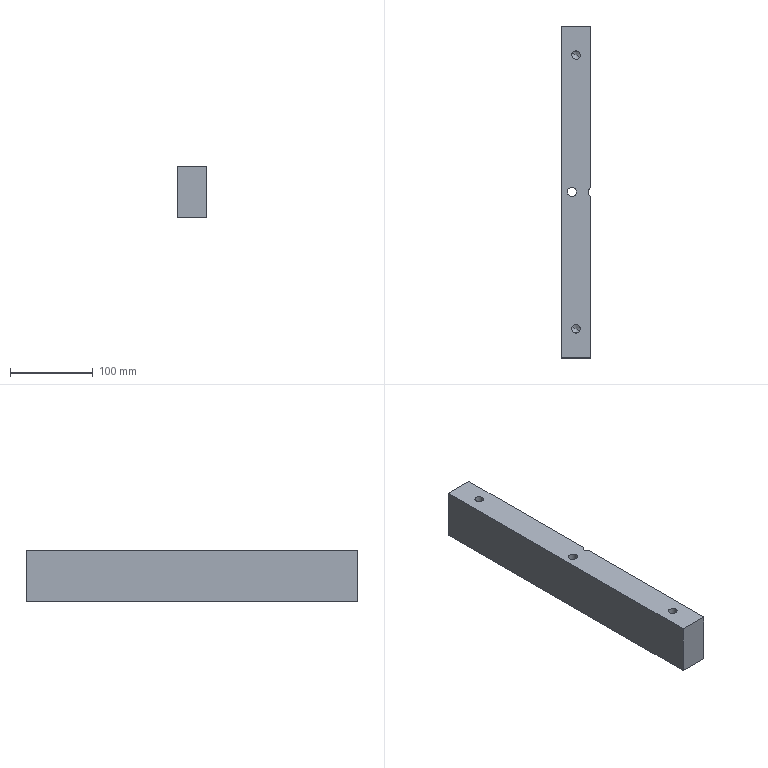Part | CATIA | 1 solid | 31 faces | box 35 x 400 x 61.7 mm | volume 841945 mm3 | cylinder 14 | cone 10 | plane 7 | commonest cylinder face diameters 10.2 x10 11 x4
STEP:
#1=CARTESIAN_POINT('',(-17.5,200.,-275.));
#2=VERTEX_POINT('',#1);
#3=CARTESIAN_POINT('',(-17.5,-200.,-275.));
#4=VERTEX_POINT('',#3);
#5=CARTESIAN_POINT('',(-17.5,0.,-275.));
#6=DIRECTION('',(0.,-1.,0.));
#7=VECTOR('',#6,1.);
#8=LINE('',#5,#7);
#9=EDGE_CURVE('',#2,#4,#8,.T.);
#10=ORIENTED_EDGE('',*,*,#9,.T.);
#11=CARTESIAN_POINT('',(-17.5,-200.,-213.3));
#12=VERTEX_POINT('',#11);
#13=CARTESIAN_POINT('',(-17.5,-200.,-244.15));
#14=DIRECTION('',(0.,0.,-1.));
#15=VECTOR('',#14,1.);
#16=LINE('',#13,#15);
#17=EDGE_CURVE('',#12,#4,#16,.T.);
#18=ORIENTED_EDGE('',*,*,#17,.F.);
#19=CARTESIAN_POINT('',(-17.5,200.,-213.3));
#20=VERTEX_POINT('',#19);
#21=CARTESIAN_POINT('',(-17.5,0.,-213.3));
#22=DIRECTION('',(0.,-1.,0.));
#23=VECTOR('',#22,1.);
#24=LINE('',#21,#23);
#25=EDGE_CURVE('',#20,#12,#24,.T.);
#26=ORIENTED_EDGE('',*,*,#25,.F.);
#27=CARTESIAN_POINT('',(-17.5,200.,-244.15));
#28=DIRECTION('',(0.,0.,-1.));
#29=VECTOR('',#28,1.);
#30=LINE('',#27,#29);
#31=EDGE_CURVE('',#20,#2,#30,.T.);
#32=ORIENTED_EDGE('',*,*,#31,.T.);
#33=EDGE_LOOP('',(#10,#18,#26,#32));
#34=FACE_OUTER_BOUND('',#33,.T.);
#35=CARTESIAN_POINT('',(-17.5,200.,0.));
#36=DIRECTION('',(1.,0.,0.));
#37=DIRECTION('',(0.,-1.,0.));
#38=AXIS2_PLACEMENT_3D('',#35,#36,#37);
#39=PLANE('',#38);
#40=ADVANCED_FACE('',(#34),#39,.F.);
#41=CARTESIAN_POINT('',(17.5,-200.,-275.));
#42=VERTEX_POINT('',#41);
#43=CARTESIAN_POINT('',(0.,-200.,-275.));
#44=DIRECTION('',(-1.,0.,0.));
#45=VECTOR('',#44,1.);
#46=LINE('',#43,#45);
#47=EDGE_CURVE('',#4,#42,#46,.F.);
#48=ORIENTED_EDGE('',*,*,#47,.T.);
#49=CARTESIAN_POINT('',(17.5,-200.,-213.3));
#50=VERTEX_POINT('',#49);
#51=CARTESIAN_POINT('',(17.5,-200.,-244.15));
#52=DIRECTION('',(0.,0.,-1.));
#53=VECTOR('',#52,1.);
#54=LINE('',#51,#53);
#55=EDGE_CURVE('',#50,#42,#54,.T.);
#56=ORIENTED_EDGE('',*,*,#55,.F.);
#57=CARTESIAN_POINT('',(0.,-200.,-213.3));
#58=DIRECTION('',(-1.,0.,0.));
#59=VECTOR('',#58,1.);
#60=LINE('',#57,#59);
#61=EDGE_CURVE('',#12,#50,#60,.F.);
#62=ORIENTED_EDGE('',*,*,#61,.F.);
#63=ORIENTED_EDGE('',*,*,#17,.T.);
#64=EDGE_LOOP('',(#48,#56,#62,#63));
#65=FACE_OUTER_BOUND('',#64,.T.);
#66=CARTESIAN_POINT('',(17.5,-200.,0.));
#67=DIRECTION('',(0.,-1.,0.));
#68=DIRECTION('',(-1.,0.,0.));
#69=AXIS2_PLACEMENT_3D('',#66,#67,#68);
#70=PLANE('',#69);
#71=ADVANCED_FACE('',(#65),#70,.T.);
#72=CARTESIAN_POINT('',(17.5,200.,-275.));
#73=VERTEX_POINT('',#72);
#74=CARTESIAN_POINT('',(0.,200.,-275.));
#75=DIRECTION('',(1.,0.,0.));
#76=VECTOR('',#75,1.);
#77=LINE('',#74,#76);
#78=EDGE_CURVE('',#73,#2,#77,.F.);
#79=ORIENTED_EDGE('',*,*,#78,.T.);
#80=ORIENTED_EDGE('',*,*,#31,.F.);
#81=CARTESIAN_POINT('',(17.5,200.,-213.3));
#82=VERTEX_POINT('',#81);
#83=CARTESIAN_POINT('',(0.,200.,-213.3));
#84=DIRECTION('',(1.,0.,0.));
#85=VECTOR('',#84,1.);
#86=LINE('',#83,#85);
#87=EDGE_CURVE('',#82,#20,#86,.F.);
#88=ORIENTED_EDGE('',*,*,#87,.F.);
#89=CARTESIAN_POINT('',(17.5,200.,-244.15));
#90=DIRECTION('',(0.,0.,-1.));
#91=VECTOR('',#90,1.);
#92=LINE('',#89,#91);
#93=EDGE_CURVE('',#82,#73,#92,.T.);
#94=ORIENTED_EDGE('',*,*,#93,.T.);
#95=EDGE_LOOP('',(#79,#80,#88,#94));
#96=FACE_OUTER_BOUND('',#95,.T.);
#97=CARTESIAN_POINT('',(-17.5,200.,0.));
#98=DIRECTION('',(0.,1.,0.));
#99=DIRECTION('',(1.,0.,0.));
#100=AXIS2_PLACEMENT_3D('',#97,#98,#99);
#101=PLANE('',#100);
#102=ADVANCED_FACE('',(#96),#101,.T.);
#103=CARTESIAN_POINT('',(17.5,4.899,-213.3));
#104=VERTEX_POINT('',#103);
#105=CARTESIAN_POINT('',(17.5,4.899,-275.));
#106=VERTEX_POINT('',#105);
#107=CARTESIAN_POINT('',(17.5,4.899,-244.15));
#108=DIRECTION('',(0.,0.,-1.));
#109=VECTOR('',#108,1.);
#110=LINE('',#107,#109);
#111=EDGE_CURVE('',#104,#106,#110,.T.);
#112=ORIENTED_EDGE('',*,*,#111,.T.);
#113=CARTESIAN_POINT('',(17.5,102.449,-275.));
#114=DIRECTION('',(0.,1.,0.));
#115=VECTOR('',#114,1.);
#116=LINE('',#113,#115);
#117=EDGE_CURVE('',#106,#73,#116,.T.);
#118=ORIENTED_EDGE('',*,*,#117,.T.);
#119=ORIENTED_EDGE('',*,*,#93,.F.);
#120=CARTESIAN_POINT('',(17.5,102.449,-213.3));
#121=DIRECTION('',(0.,1.,0.));
#122=VECTOR('',#121,1.);
#123=LINE('',#120,#122);
#124=EDGE_CURVE('',#104,#82,#123,.T.);
#125=ORIENTED_EDGE('',*,*,#124,.F.);
#126=EDGE_LOOP('',(#112,#118,#119,#125));
#127=FACE_OUTER_BOUND('',#126,.T.);
#128=CARTESIAN_POINT('',(17.5,-200.,0.));
#129=DIRECTION('',(-1.,0.,0.));
#130=DIRECTION('',(0.,1.,0.));
#131=AXIS2_PLACEMENT_3D('',#128,#129,#130);
#132=PLANE('',#131);
#133=ADVANCED_FACE('',(#127),#132,.F.);
#134=CARTESIAN_POINT('',(17.5,-4.899,-213.3));
#135=VERTEX_POINT('',#134);
#136=CARTESIAN_POINT('',(17.5,-4.899,-275.));
#137=VERTEX_POINT('',#136);
#138=CARTESIAN_POINT('',(17.5,-4.899,-244.15));
#139=DIRECTION('',(0.,0.,-1.));
#140=VECTOR('',#139,1.);
#141=LINE('',#138,#140);
#142=EDGE_CURVE('',#135,#137,#141,.T.);
#143=ORIENTED_EDGE('',*,*,#142,.F.);
#144=CARTESIAN_POINT('',(17.5,-102.449,-213.3));
#145=DIRECTION('',(0.,1.,0.));
#146=VECTOR('',#145,1.);
#147=LINE('',#144,#146);
#148=EDGE_CURVE('',#50,#135,#147,.T.);
#149=ORIENTED_EDGE('',*,*,#148,.F.);
#150=ORIENTED_EDGE('',*,*,#55,.T.);
#151=CARTESIAN_POINT('',(17.5,-102.449,-275.));
#152=DIRECTION('',(0.,1.,0.));
#153=VECTOR('',#152,1.);
#154=LINE('',#151,#153);
#155=EDGE_CURVE('',#42,#137,#154,.T.);
#156=ORIENTED_EDGE('',*,*,#155,.T.);
#157=EDGE_LOOP('',(#143,#149,#150,#156));
#158=FACE_OUTER_BOUND('',#157,.T.);
#159=ADVANCED_FACE('',(#158),#132,.F.);
#160=CARTESIAN_POINT('',(15.173,2.637,-213.3));
#161=VERTEX_POINT('',#160);
#162=CARTESIAN_POINT('',(20.,0.,-213.3));
#163=DIRECTION('',(0.,0.,-1.));
#164=AXIS2_PLACEMENT_3D('',#162,#163,$);
#165=CIRCLE('',#164,5.5);
#166=EDGE_CURVE('',#161,#135,#165,.F.);
#167=ORIENTED_EDGE('',*,*,#166,.T.);
#168=ORIENTED_EDGE('',*,*,#142,.T.);
#169=CARTESIAN_POINT('',(15.173,2.637,-275.));
#170=VERTEX_POINT('',#169);
#171=CARTESIAN_POINT('',(20.,0.,-275.));
#172=DIRECTION('',(0.,0.,-1.));
#173=AXIS2_PLACEMENT_3D('',#171,#172,$);
#174=CIRCLE('',#173,5.5);
#175=EDGE_CURVE('',#170,#137,#174,.F.);
#176=ORIENTED_EDGE('',*,*,#175,.F.);
#177=CARTESIAN_POINT('',(15.173,2.637,-270.8));
#178=DIRECTION('',(0.,0.,-1.));
#179=VECTOR('',#178,1.);
#180=LINE('',#177,#179);
#181=EDGE_CURVE('',#170,#161,#180,.F.);
#182=ORIENTED_EDGE('',*,*,#181,.T.);
#183=EDGE_LOOP('',(#167,#168,#176,#182));
#184=FACE_OUTER_BOUND('',#183,.T.);
#185=CARTESIAN_POINT('',(20.,0.,-196.1));
#186=DIRECTION('',(0.,0.,-1.));
#187=DIRECTION('',(0.8776,-0.4794,0.));
#188=AXIS2_PLACEMENT_3D('',#185,#186,#187);
#189=CYLINDRICAL_SURFACE('',#188,5.5);
#190=ADVANCED_FACE('',(#184),#189,.F.);
#191=CARTESIAN_POINT('',(20.,0.,-275.));
#192=DIRECTION('',(0.,0.,-1.));
#193=AXIS2_PLACEMENT_3D('',#191,#192,$);
#194=CIRCLE('',#193,5.5);
#195=EDGE_CURVE('',#106,#170,#194,.F.);
#196=ORIENTED_EDGE('',*,*,#195,.F.);
#197=ORIENTED_EDGE('',*,*,#111,.F.);
#198=CARTESIAN_POINT('',(20.,0.,-213.3));
#199=DIRECTION('',(0.,0.,-1.));
#200=AXIS2_PLACEMENT_3D('',#198,#199,$);
#201=CIRCLE('',#200,5.5);
#202=EDGE_CURVE('',#104,#161,#201,.F.);
#203=ORIENTED_EDGE('',*,*,#202,.T.);
#204=ORIENTED_EDGE('',*,*,#181,.F.);
#205=EDGE_LOOP('',(#196,#197,#203,#204));
#206=FACE_OUTER_BOUND('',#205,.T.);
#207=ADVANCED_FACE('',(#206),#189,.F.);
#208=CARTESIAN_POINT('',(-9.827,2.637,-275.));
#209=VERTEX_POINT('',#208);
#210=CARTESIAN_POINT('',(-9.827,2.637,-213.3));
#211=VERTEX_POINT('',#210);
#212=CARTESIAN_POINT('',(-9.827,2.637,-270.8));
#213=DIRECTION('',(0.,0.,-1.));
#214=VECTOR('',#213,1.);
#215=LINE('',#212,#214);
#216=EDGE_CURVE('',#209,#211,#215,.F.);
#217=ORIENTED_EDGE('',*,*,#216,.T.);
#218=CARTESIAN_POINT('',(-0.1733,-2.637,-213.3));
#219=VERTEX_POINT('',#218);
#220=CARTESIAN_POINT('',(-5.,0.,-213.3));
#221=DIRECTION('',(0.,0.,-1.));
#222=AXIS2_PLACEMENT_3D('',#220,#221,$);
#223=CIRCLE('',#222,5.5);
#224=EDGE_CURVE('',#211,#219,#223,.F.);
#225=ORIENTED_EDGE('',*,*,#224,.T.);
#226=CARTESIAN_POINT('',(-0.1733,-2.637,-275.));
#227=VERTEX_POINT('',#226);
#228=CARTESIAN_POINT('',(-0.1733,-2.637,-270.8));
#229=DIRECTION('',(0.,0.,-1.));
#230=VECTOR('',#229,1.);
#231=LINE('',#228,#230);
#232=EDGE_CURVE('',#227,#219,#231,.F.);
#233=ORIENTED_EDGE('',*,*,#232,.F.);
#234=CARTESIAN_POINT('',(-5.,0.,-275.));
#235=DIRECTION('',(0.,0.,-1.));
#236=AXIS2_PLACEMENT_3D('',#234,#235,$);
#237=CIRCLE('',#236,5.5);
#238=EDGE_CURVE('',#209,#227,#237,.F.);
#239=ORIENTED_EDGE('',*,*,#238,.F.);
#240=EDGE_LOOP('',(#217,#225,#233,#239));
#241=FACE_OUTER_BOUND('',#240,.T.);
#242=CARTESIAN_POINT('',(-5.,0.,-196.1));
#243=DIRECTION('',(0.,0.,-1.));
#244=DIRECTION('',(0.8776,-0.4794,0.));
#245=AXIS2_PLACEMENT_3D('',#242,#243,#244);
#246=CYLINDRICAL_SURFACE('',#245,5.5);
#247=ADVANCED_FACE('',(#241),#246,.F.);
#248=ORIENTED_EDGE('',*,*,#232,.T.);
#249=CARTESIAN_POINT('',(-5.,0.,-213.3));
#250=DIRECTION('',(0.,0.,-1.));
#251=AXIS2_PLACEMENT_3D('',#249,#250,$);
#252=CIRCLE('',#251,5.5);
#253=EDGE_CURVE('',#219,#211,#252,.F.);
#254=ORIENTED_EDGE('',*,*,#253,.T.);
#255=ORIENTED_EDGE('',*,*,#216,.F.);
#256=CARTESIAN_POINT('',(-5.,0.,-275.));
#257=DIRECTION('',(0.,0.,-1.));
#258=AXIS2_PLACEMENT_3D('',#256,#257,$);
#259=CIRCLE('',#258,5.5);
#260=EDGE_CURVE('',#227,#209,#259,.F.);
#261=ORIENTED_EDGE('',*,*,#260,.F.);
#262=EDGE_LOOP('',(#248,#254,#255,#261));
#263=FACE_OUTER_BOUND('',#262,.T.);
#264=ADVANCED_FACE('',(#263),#246,.F.);
#265=ORIENTED_EDGE('',*,*,#124,.T.);
#266=ORIENTED_EDGE('',*,*,#87,.T.);
#267=ORIENTED_EDGE('',*,*,#25,.T.);
#268=ORIENTED_EDGE('',*,*,#61,.T.);
#269=ORIENTED_EDGE('',*,*,#148,.T.);
#270=ORIENTED_EDGE('',*,*,#166,.F.);
#271=ORIENTED_EDGE('',*,*,#202,.F.);
#272=EDGE_LOOP('',(#265,#266,#267,#268,#269,#270,#271));
#273=FACE_OUTER_BOUND('',#272,.T.);
#274=ORIENTED_EDGE('',*,*,#253,.F.);
#275=ORIENTED_EDGE('',*,*,#224,.F.);
#276=EDGE_LOOP('',(#274,#275));
#277=FACE_BOUND('',#276,.T.);
#278=CARTESIAN_POINT('',(4.476,162.555,-213.3));
#279=VERTEX_POINT('',#278);
#280=CARTESIAN_POINT('',(-4.476,167.445,-213.3));
#281=VERTEX_POINT('',#280);
#282=CARTESIAN_POINT('',(0.,165.,-213.3));
#283=DIRECTION('',(0.,0.,1.));
#284=AXIS2_PLACEMENT_3D('',#282,#283,$);
#285=CIRCLE('',#284,5.1);
#286=EDGE_CURVE('',#279,#281,#285,.T.);
#287=ORIENTED_EDGE('',*,*,#286,.F.);
#288=CARTESIAN_POINT('',(0.,165.,-213.3));
#289=DIRECTION('',(0.,0.,1.));
#290=AXIS2_PLACEMENT_3D('',#288,#289,$);
#291=CIRCLE('',#290,5.1);
#292=EDGE_CURVE('',#281,#279,#291,.T.);
#293=ORIENTED_EDGE('',*,*,#292,.F.);
#294=EDGE_LOOP('',(#287,#293));
#295=FACE_BOUND('',#294,.T.);
#296=CARTESIAN_POINT('',(4.476,-167.445,-213.3));
#297=VERTEX_POINT('',#296);
#298=CARTESIAN_POINT('',(-4.476,-162.555,-213.3));
#299=VERTEX_POINT('',#298);
#300=CARTESIAN_POINT('',(0.,-165.,-213.3));
#301=DIRECTION('',(0.,0.,1.));
#302=AXIS2_PLACEMENT_3D('',#300,#301,$);
#303=CIRCLE('',#302,5.1);
#304=EDGE_CURVE('',#297,#299,#303,.T.);
#305=ORIENTED_EDGE('',*,*,#304,.F.);
#306=CARTESIAN_POINT('',(0.,-165.,-213.3));
#307=DIRECTION('',(0.,0.,1.));
#308=AXIS2_PLACEMENT_3D('',#306,#307,$);
#309=CIRCLE('',#308,5.1);
#310=EDGE_CURVE('',#299,#297,#309,.T.);
#311=ORIENTED_EDGE('',*,*,#310,.F.);
#312=EDGE_LOOP('',(#305,#311));
#313=FACE_BOUND('',#312,.T.);
#314=CARTESIAN_POINT('',(0.,0.,-213.3));
#315=DIRECTION('',(0.,0.,1.));
#316=DIRECTION('',(1.,0.,0.));
#317=AXIS2_PLACEMENT_3D('',#314,#315,#316);
#318=PLANE('',#317);
#319=ADVANCED_FACE('',(#273,#277,#295,#313),#318,.T.);
#320=ORIENTED_EDGE('',*,*,#195,.T.);
#321=ORIENTED_EDGE('',*,*,#175,.T.);
#322=ORIENTED_EDGE('',*,*,#155,.F.);
#323=ORIENTED_EDGE('',*,*,#47,.F.);
#324=ORIENTED_EDGE('',*,*,#9,.F.);
#325=ORIENTED_EDGE('',*,*,#78,.F.);
#326=ORIENTED_EDGE('',*,*,#117,.F.);
#327=EDGE_LOOP('',(#320,#321,#322,#323,#324,#325,#326));
#328=FACE_OUTER_BOUND('',#327,.T.);
#329=ORIENTED_EDGE('',*,*,#238,.T.);
#330=ORIENTED_EDGE('',*,*,#260,.T.);
#331=EDGE_LOOP('',(#329,#330));
#332=FACE_BOUND('',#331,.T.);
#333=CARTESIAN_POINT('',(4.476,177.445,-275.));
#334=VERTEX_POINT('',#333);
#335=CARTESIAN_POINT('',(-4.476,172.555,-275.));
#336=VERTEX_POINT('',#335);
#337=CARTESIAN_POINT('',(0.,175.,-275.));
#338=DIRECTION('',(0.,0.,1.));
#339=AXIS2_PLACEMENT_3D('',#337,#338,$);
#340=CIRCLE('',#339,5.1);
#341=EDGE_CURVE('',#334,#336,#340,.T.);
#342=ORIENTED_EDGE('',*,*,#341,.T.);
#343=CARTESIAN_POINT('',(0.,175.,-275.));
#344=DIRECTION('',(0.,0.,1.));
#345=AXIS2_PLACEMENT_3D('',#343,#344,$);
#346=CIRCLE('',#345,5.1);
#347=EDGE_CURVE('',#336,#334,#346,.T.);
#348=ORIENTED_EDGE('',*,*,#347,.T.);
#349=EDGE_LOOP('',(#342,#348));
#350=FACE_BOUND('',#349,.T.);
#351=CARTESIAN_POINT('',(4.476,-172.555,-275.));
#352=VERTEX_POINT('',#351);
#353=CARTESIAN_POINT('',(-4.476,-177.445,-275.));
#354=VERTEX_POINT('',#353);
#355=CARTESIAN_POINT('',(0.,-175.,-275.));
#356=DIRECTION('',(0.,0.,1.));
#357=AXIS2_PLACEMENT_3D('',#355,#356,$);
#358=CIRCLE('',#357,5.1);
#359=EDGE_CURVE('',#352,#354,#358,.T.);
#360=ORIENTED_EDGE('',*,*,#359,.T.);
#361=CARTESIAN_POINT('',(0.,-175.,-275.));
#362=DIRECTION('',(0.,0.,1.));
#363=AXIS2_PLACEMENT_3D('',#361,#362,$);
#364=CIRCLE('',#363,5.1);
#365=EDGE_CURVE('',#354,#352,#364,.T.);
#366=ORIENTED_EDGE('',*,*,#365,.T.);
#367=EDGE_LOOP('',(#360,#366));
#368=FACE_BOUND('',#367,.T.);
#369=CARTESIAN_POINT('',(4.476,-37.555,-275.));
#370=VERTEX_POINT('',#369);
#371=CARTESIAN_POINT('',(-4.476,-42.445,-275.));
#372=VERTEX_POINT('',#371);
#373=CARTESIAN_POINT('',(0.,-40.,-275.));
#374=DIRECTION('',(0.,0.,1.));
#375=AXIS2_PLACEMENT_3D('',#373,#374,$);
#376=CIRCLE('',#375,5.1);
#377=EDGE_CURVE('',#370,#372,#376,.T.);
#378=ORIENTED_EDGE('',*,*,#377,.T.);
#379=CARTESIAN_POINT('',(0.,-40.,-275.));
#380=DIRECTION('',(0.,0.,1.));
#381=AXIS2_PLACEMENT_3D('',#379,#380,$);
#382=CIRCLE('',#381,5.1);
#383=EDGE_CURVE('',#372,#370,#382,.T.);
#384=ORIENTED_EDGE('',*,*,#383,.T.);
#385=EDGE_LOOP('',(#378,#384));
#386=FACE_BOUND('',#385,.T.);
#387=CARTESIAN_POINT('',(0.,0.,-275.));
#388=DIRECTION('',(0.,0.,1.));
#389=DIRECTION('',(1.,0.,0.));
#390=AXIS2_PLACEMENT_3D('',#387,#388,#389);
#391=PLANE('',#390);
#392=ADVANCED_FACE('',(#328,#332,#350,#368,#386),#391,.F.);
#393=CARTESIAN_POINT('',(0.,-40.,-237.056));
#394=VERTEX_POINT('',#393);
#395=CARTESIAN_POINT('',(-4.476,-42.445,-240.));
#396=VERTEX_POINT('',#395);
#397=CARTESIAN_POINT('',(-2.238,-41.223,-238.528));
#398=DIRECTION('',(-0.76,-0.4152,-0.5));
#399=VECTOR('',#398,1.);
#400=LINE('',#397,#399);
#401=EDGE_CURVE('',#394,#396,#400,.T.);
#402=ORIENTED_EDGE('',*,*,#401,.T.);
#403=CARTESIAN_POINT('',(4.476,-37.555,-240.));
#404=VERTEX_POINT('',#403);
#405=CARTESIAN_POINT('',(0.,-40.,-240.));
#406=DIRECTION('',(0.,0.,-1.));
#407=AXIS2_PLACEMENT_3D('',#405,#406,$);
#408=CIRCLE('',#407,5.1);
#409=EDGE_CURVE('',#404,#396,#408,.F.);
#410=ORIENTED_EDGE('',*,*,#409,.F.);
#411=CARTESIAN_POINT('',(2.238,-38.777,-238.528));
#412=DIRECTION('',(0.76,0.4152,-0.5));
#413=VECTOR('',#412,1.);
#414=LINE('',#411,#413);
#415=EDGE_CURVE('',#394,#404,#414,.T.);
#416=ORIENTED_EDGE('',*,*,#415,.F.);
#417=EDGE_LOOP('',(#402,#410,#416));
#418=FACE_OUTER_BOUND('',#417,.T.);
#419=CARTESIAN_POINT('',(0.,-40.,-237.056));
#420=DIRECTION('',(0.,0.,-1.));
#421=DIRECTION('',(0.8776,0.4794,0.));
#422=AXIS2_PLACEMENT_3D('',#419,#420,#421);
#423=CONICAL_SURFACE('',#422,0.,1.047);
#424=ADVANCED_FACE('',(#418),#423,.F.);
#425=ORIENTED_EDGE('',*,*,#415,.T.);
#426=CARTESIAN_POINT('',(0.,-40.,-240.));
#427=DIRECTION('',(0.,0.,-1.));
#428=AXIS2_PLACEMENT_3D('',#426,#427,$);
#429=CIRCLE('',#428,5.1);
#430=EDGE_CURVE('',#396,#404,#429,.F.);
#431=ORIENTED_EDGE('',*,*,#430,.F.);
#432=ORIENTED_EDGE('',*,*,#401,.F.);
#433=EDGE_LOOP('',(#425,#431,#432));
#434=FACE_OUTER_BOUND('',#433,.T.);
#435=ADVANCED_FACE('',(#434),#423,.F.);
#436=ORIENTED_EDGE('',*,*,#377,.F.);
#437=CARTESIAN_POINT('',(4.476,-37.555,-257.7));
#438=DIRECTION('',(0.,0.,1.));
#439=VECTOR('',#438,1.);
#440=LINE('',#437,#439);
#441=EDGE_CURVE('',#404,#370,#440,.F.);
#442=ORIENTED_EDGE('',*,*,#441,.F.);
#443=ORIENTED_EDGE('',*,*,#409,.T.);
#444=CARTESIAN_POINT('',(-4.476,-42.445,-257.7));
#445=DIRECTION('',(0.,0.,1.));
#446=VECTOR('',#445,1.);
#447=LINE('',#444,#446);
#448=EDGE_CURVE('',#396,#372,#447,.F.);
#449=ORIENTED_EDGE('',*,*,#448,.T.);
#450=EDGE_LOOP('',(#436,#442,#443,#449));
#451=FACE_OUTER_BOUND('',#450,.T.);
#452=CARTESIAN_POINT('',(0.,-40.,-274.9));
#453=DIRECTION('',(0.,0.,1.));
#454=DIRECTION('',(0.8776,0.4794,0.));
#455=AXIS2_PLACEMENT_3D('',#452,#453,#454);
#456=CYLINDRICAL_SURFACE('',#455,5.1);
#457=ADVANCED_FACE('',(#451),#456,.F.);
#458=ORIENTED_EDGE('',*,*,#383,.F.);
#459=ORIENTED_EDGE('',*,*,#448,.F.);
#460=ORIENTED_EDGE('',*,*,#430,.T.);
#461=ORIENTED_EDGE('',*,*,#441,.T.);
#462=EDGE_LOOP('',(#458,#459,#460,#461));
#463=FACE_OUTER_BOUND('',#462,.T.);
#464=ADVANCED_FACE('',(#463),#456,.F.);
#465=CARTESIAN_POINT('',(0.,-165.,-251.244));
#466=VERTEX_POINT('',#465);
#467=CARTESIAN_POINT('',(4.476,-167.445,-248.3));
#468=VERTEX_POINT('',#467);
#469=CARTESIAN_POINT('',(2.238,-166.223,-249.772));
#470=DIRECTION('',(0.76,-0.4152,0.5));
#471=VECTOR('',#470,1.);
#472=LINE('',#469,#471);
#473=EDGE_CURVE('',#466,#468,#472,.T.);
#474=ORIENTED_EDGE('',*,*,#473,.T.);
#475=CARTESIAN_POINT('',(-4.476,-162.555,-248.3));
#476=VERTEX_POINT('',#475);
#477=CARTESIAN_POINT('',(0.,-165.,-248.3));
#478=DIRECTION('',(0.,0.,1.));
#479=AXIS2_PLACEMENT_3D('',#477,#478,$);
#480=CIRCLE('',#479,5.1);
#481=EDGE_CURVE('',#476,#468,#480,.F.);
#482=ORIENTED_EDGE('',*,*,#481,.F.);
#483=CARTESIAN_POINT('',(-2.238,-163.777,-249.772));
#484=DIRECTION('',(-0.76,0.4152,0.5));
#485=VECTOR('',#484,1.);
#486=LINE('',#483,#485);
#487=EDGE_CURVE('',#466,#476,#486,.T.);
#488=ORIENTED_EDGE('',*,*,#487,.F.);
#489=EDGE_LOOP('',(#474,#482,#488));
#490=FACE_OUTER_BOUND('',#489,.T.);
#491=CARTESIAN_POINT('',(0.,-165.,-251.244));
#492=DIRECTION('',(0.,0.,1.));
#493=DIRECTION('',(0.8776,-0.4794,0.));
#494=AXIS2_PLACEMENT_3D('',#491,#492,#493);
#495=CONICAL_SURFACE('',#494,0.,1.047);
#496=ADVANCED_FACE('',(#490),#495,.F.);
#497=CARTESIAN_POINT('',(-1.005,-170.,-248.3));
#498=VERTEX_POINT('',#497);
#499=CARTESIAN_POINT('',(1.005,-170.,-248.3));
#500=VERTEX_POINT('',#499);
#501=CARTESIAN_POINT('',(-1.005,-170.,-248.3));
#502=CARTESIAN_POINT('',(-0.6257,-169.924,-248.386));
#503=CARTESIAN_POINT('',(-0.2179,-169.878,-248.441));
#504=CARTESIAN_POINT('',(0.2179,-169.878,-248.441));
#505=CARTESIAN_POINT('',(0.6257,-169.924,-248.386));
#506=CARTESIAN_POINT('',(1.005,-170.,-248.3));
#507=B_SPLINE_CURVE_WITH_KNOTS('',5,(#501,#502,#503,#504,#505,#506),.UNSPECIFIED.,.F.,.U.,(6,6),(0.,2.339),.UNSPECIFIED.);
#508=EDGE_CURVE('',#498,#500,#507,.T.);
#509=ORIENTED_EDGE('',*,*,#508,.T.);
#510=CARTESIAN_POINT('',(0.,-165.,-248.3));
#511=DIRECTION('',(0.,0.,1.));
#512=AXIS2_PLACEMENT_3D('',#510,#511,$);
#513=CIRCLE('',#512,5.1);
#514=EDGE_CURVE('',#468,#500,#513,.F.);
#515=ORIENTED_EDGE('',*,*,#514,.F.);
#516=ORIENTED_EDGE('',*,*,#473,.F.);
#517=ORIENTED_EDGE('',*,*,#487,.T.);
#518=CARTESIAN_POINT('',(0.,-165.,-248.3));
#519=DIRECTION('',(0.,0.,1.));
#520=AXIS2_PLACEMENT_3D('',#518,#519,$);
#521=CIRCLE('',#520,5.1);
#522=EDGE_CURVE('',#498,#476,#521,.F.);
#523=ORIENTED_EDGE('',*,*,#522,.F.);
#524=EDGE_LOOP('',(#509,#515,#516,#517,#523));
#525=FACE_OUTER_BOUND('',#524,.T.);
#526=ADVANCED_FACE('',(#525),#495,.F.);
#527=ORIENTED_EDGE('',*,*,#304,.T.);
#528=CARTESIAN_POINT('',(-4.476,-162.555,-230.6));
#529=DIRECTION('',(0.,0.,-1.));
#530=VECTOR('',#529,1.);
#531=LINE('',#528,#530);
#532=EDGE_CURVE('',#476,#299,#531,.F.);
#533=ORIENTED_EDGE('',*,*,#532,.F.);
#534=ORIENTED_EDGE('',*,*,#481,.T.);
#535=CARTESIAN_POINT('',(4.476,-167.445,-230.6));
#536=DIRECTION('',(0.,0.,-1.));
#537=VECTOR('',#536,1.);
#538=LINE('',#535,#537);
#539=EDGE_CURVE('',#468,#297,#538,.F.);
#540=ORIENTED_EDGE('',*,*,#539,.T.);
#541=EDGE_LOOP('',(#527,#533,#534,#540));
#542=FACE_OUTER_BOUND('',#541,.T.);
#543=CARTESIAN_POINT('',(0.,-165.,-213.4));
#544=DIRECTION('',(0.,0.,-1.));
#545=DIRECTION('',(0.8776,-0.4794,0.));
#546=AXIS2_PLACEMENT_3D('',#543,#544,#545);
#547=CYLINDRICAL_SURFACE('',#546,5.1);
#548=ADVANCED_FACE('',(#542),#547,.F.);
#549=CARTESIAN_POINT('',(1.005,-170.,-240.));
#550=VERTEX_POINT('',#549);
#551=CARTESIAN_POINT('',(1.005,-170.,-230.6));
#552=DIRECTION('',(0.,0.,-1.));
#553=VECTOR('',#552,1.);
#554=LINE('',#551,#553);
#555=EDGE_CURVE('',#550,#500,#554,.T.);
#556=ORIENTED_EDGE('',*,*,#555,.F.);
#557=CARTESIAN_POINT('',(-1.005,-170.,-240.));
#558=VERTEX_POINT('',#557);
#559=CARTESIAN_POINT('',(-1.005,-170.,-240.));
#560=CARTESIAN_POINT('',(-0.6257,-170.076,-239.914));
#561=CARTESIAN_POINT('',(-0.218,-170.122,-239.859));
#562=CARTESIAN_POINT('',(0.218,-170.122,-239.859));
#563=CARTESIAN_POINT('',(0.6257,-170.076,-239.914));
#564=CARTESIAN_POINT('',(1.005,-170.,-240.));
#565=B_SPLINE_CURVE_WITH_KNOTS('',5,(#559,#560,#561,#562,#563,#564),.UNSPECIFIED.,.F.,.U.,(6,6),(0.,2.339),.UNSPECIFIED.);
#566=EDGE_CURVE('',#558,#550,#565,.T.);
#567=ORIENTED_EDGE('',*,*,#566,.F.);
#568=CARTESIAN_POINT('',(-1.005,-170.,-230.6));
#569=DIRECTION('',(0.,0.,-1.));
#570=VECTOR('',#569,1.);
#571=LINE('',#568,#570);
#572=EDGE_CURVE('',#558,#498,#571,.T.);
#573=ORIENTED_EDGE('',*,*,#572,.T.);
#574=ORIENTED_EDGE('',*,*,#522,.T.);
#575=ORIENTED_EDGE('',*,*,#532,.T.);
#576=ORIENTED_EDGE('',*,*,#310,.T.);
#577=ORIENTED_EDGE('',*,*,#539,.F.);
#578=ORIENTED_EDGE('',*,*,#514,.T.);
#579=EDGE_LOOP('',(#556,#567,#573,#574,#575,#576,#577,#578));
#580=FACE_OUTER_BOUND('',#579,.T.);
#581=ADVANCED_FACE('',(#580),#547,.F.);
#582=ORIENTED_EDGE('',*,*,#555,.T.);
#583=ORIENTED_EDGE('',*,*,#508,.F.);
#584=ORIENTED_EDGE('',*,*,#572,.F.);
#585=CARTESIAN_POINT('',(-4.476,-177.445,-240.));
#586=VERTEX_POINT('',#585);
#587=CARTESIAN_POINT('',(0.,-175.,-240.));
#588=DIRECTION('',(0.,0.,1.));
#589=AXIS2_PLACEMENT_3D('',#587,#588,$);
#590=CIRCLE('',#589,5.1);
#591=EDGE_CURVE('',#558,#586,#590,.T.);
#592=ORIENTED_EDGE('',*,*,#591,.T.);
#593=CARTESIAN_POINT('',(-4.476,-177.445,-257.7));
#594=DIRECTION('',(0.,0.,1.));
#595=VECTOR('',#594,1.);
#596=LINE('',#593,#595);
#597=EDGE_CURVE('',#586,#354,#596,.F.);
#598=ORIENTED_EDGE('',*,*,#597,.T.);
#599=ORIENTED_EDGE('',*,*,#359,.F.);
#600=CARTESIAN_POINT('',(4.476,-172.555,-240.));
#601=VERTEX_POINT('',#600);
#602=CARTESIAN_POINT('',(4.476,-172.555,-257.7));
#603=DIRECTION('',(0.,0.,1.));
#604=VECTOR('',#603,1.);
#605=LINE('',#602,#604);
#606=EDGE_CURVE('',#601,#352,#605,.F.);
#607=ORIENTED_EDGE('',*,*,#606,.F.);
#608=CARTESIAN_POINT('',(0.,-175.,-240.));
#609=DIRECTION('',(0.,0.,1.));
#610=AXIS2_PLACEMENT_3D('',#608,#609,$);
#611=CIRCLE('',#610,5.1);
#612=EDGE_CURVE('',#601,#550,#611,.T.);
#613=ORIENTED_EDGE('',*,*,#612,.T.);
#614=EDGE_LOOP('',(#582,#583,#584,#592,#598,#599,#607,#613));
#615=FACE_OUTER_BOUND('',#614,.T.);
#616=CARTESIAN_POINT('',(0.,-175.,-274.9));
#617=DIRECTION('',(0.,0.,1.));
#618=DIRECTION('',(0.8776,0.4794,0.));
#619=AXIS2_PLACEMENT_3D('',#616,#617,#618);
#620=CYLINDRICAL_SURFACE('',#619,5.1);
#621=ADVANCED_FACE('',(#615),#620,.F.);
#622=ORIENTED_EDGE('',*,*,#566,.T.);
#623=ORIENTED_EDGE('',*,*,#612,.F.);
#624=CARTESIAN_POINT('',(0.,-175.,-237.056));
#625=VERTEX_POINT('',#624);
#626=CARTESIAN_POINT('',(2.238,-173.777,-238.528));
#627=DIRECTION('',(0.76,0.4152,-0.5));
#628=VECTOR('',#627,1.);
#629=LINE('',#626,#628);
#630=EDGE_CURVE('',#625,#601,#629,.T.);
#631=ORIENTED_EDGE('',*,*,#630,.F.);
#632=CARTESIAN_POINT('',(-2.238,-176.223,-238.528));
#633=DIRECTION('',(-0.76,-0.4152,-0.5));
#634=VECTOR('',#633,1.);
#635=LINE('',#632,#634);
#636=EDGE_CURVE('',#625,#586,#635,.T.);
#637=ORIENTED_EDGE('',*,*,#636,.T.);
#638=ORIENTED_EDGE('',*,*,#591,.F.);
#639=EDGE_LOOP('',(#622,#623,#631,#637,#638));
#640=FACE_OUTER_BOUND('',#639,.T.);
#641=CARTESIAN_POINT('',(0.,-175.,-237.056));
#642=DIRECTION('',(0.,0.,-1.));
#643=DIRECTION('',(0.8776,0.4794,0.));
#644=AXIS2_PLACEMENT_3D('',#641,#642,#643);
#645=CONICAL_SURFACE('',#644,0.,1.047);
#646=ADVANCED_FACE('',(#640),#645,.F.);
#647=ORIENTED_EDGE('',*,*,#365,.F.);
#648=ORIENTED_EDGE('',*,*,#597,.F.);
#649=CARTESIAN_POINT('',(0.,-175.,-240.));
#650=DIRECTION('',(0.,0.,1.));
#651=AXIS2_PLACEMENT_3D('',#649,#650,$);
#652=CIRCLE('',#651,5.1);
#653=EDGE_CURVE('',#586,#601,#652,.T.);
#654=ORIENTED_EDGE('',*,*,#653,.T.);
#655=ORIENTED_EDGE('',*,*,#606,.T.);
#656=EDGE_LOOP('',(#647,#648,#654,#655));
#657=FACE_OUTER_BOUND('',#656,.T.);
#658=ADVANCED_FACE('',(#657),#620,.F.);
#659=ORIENTED_EDGE('',*,*,#630,.T.);
#660=ORIENTED_EDGE('',*,*,#653,.F.);
#661=ORIENTED_EDGE('',*,*,#636,.F.);
#662=EDGE_LOOP('',(#659,#660,#661));
#663=FACE_OUTER_BOUND('',#662,.T.);
#664=ADVANCED_FACE('',(#663),#645,.F.);
#665=CARTESIAN_POINT('',(0.,165.,-251.244));
#666=VERTEX_POINT('',#665);
#667=CARTESIAN_POINT('',(-4.476,167.445,-248.3));
#668=VERTEX_POINT('',#667);
#669=CARTESIAN_POINT('',(-2.238,166.223,-249.772));
#670=DIRECTION('',(-0.76,0.4152,0.5));
#671=VECTOR('',#670,1.);
#672=LINE('',#669,#671);
#673=EDGE_CURVE('',#666,#668,#672,.T.);
#674=ORIENTED_EDGE('',*,*,#673,.T.);
#675=CARTESIAN_POINT('',(4.476,162.555,-248.3));
#676=VERTEX_POINT('',#675);
#677=CARTESIAN_POINT('',(0.,165.,-248.3));
#678=DIRECTION('',(0.,0.,1.));
#679=AXIS2_PLACEMENT_3D('',#677,#678,$);
#680=CIRCLE('',#679,5.1);
#681=EDGE_CURVE('',#676,#668,#680,.F.);
#682=ORIENTED_EDGE('',*,*,#681,.F.);
#683=CARTESIAN_POINT('',(2.238,163.777,-249.772));
#684=DIRECTION('',(0.76,-0.4152,0.5));
#685=VECTOR('',#684,1.);
#686=LINE('',#683,#685);
#687=EDGE_CURVE('',#666,#676,#686,.T.);
#688=ORIENTED_EDGE('',*,*,#687,.F.);
#689=EDGE_LOOP('',(#674,#682,#688));
#690=FACE_OUTER_BOUND('',#689,.T.);
#691=CARTESIAN_POINT('',(0.,165.,-251.244));
#692=DIRECTION('',(0.,0.,1.));
#693=DIRECTION('',(0.8776,-0.4794,0.));
#694=AXIS2_PLACEMENT_3D('',#691,#692,#693);
#695=CONICAL_SURFACE('',#694,0.,1.047);
#696=ADVANCED_FACE('',(#690),#695,.F.);
#697=CARTESIAN_POINT('',(1.005,170.,-248.3));
#698=VERTEX_POINT('',#697);
#699=CARTESIAN_POINT('',(-1.005,170.,-248.3));
#700=VERTEX_POINT('',#699);
#701=CARTESIAN_POINT('',(1.005,170.,-248.3));
#702=CARTESIAN_POINT('',(0.6257,169.924,-248.386));
#703=CARTESIAN_POINT('',(0.2179,169.878,-248.441));
#704=CARTESIAN_POINT('',(-0.2179,169.878,-248.441));
#705=CARTESIAN_POINT('',(-0.6257,169.924,-248.386));
#706=CARTESIAN_POINT('',(-1.005,170.,-248.3));
#707=B_SPLINE_CURVE_WITH_KNOTS('',5,(#701,#702,#703,#704,#705,#706),.UNSPECIFIED.,.F.,.U.,(6,6),(0.,2.339),.UNSPECIFIED.);
#708=EDGE_CURVE('',#698,#700,#707,.T.);
#709=ORIENTED_EDGE('',*,*,#708,.T.);
#710=CARTESIAN_POINT('',(0.,165.,-248.3));
#711=DIRECTION('',(0.,0.,1.));
#712=AXIS2_PLACEMENT_3D('',#710,#711,$);
#713=CIRCLE('',#712,5.1);
#714=EDGE_CURVE('',#668,#700,#713,.F.);
#715=ORIENTED_EDGE('',*,*,#714,.F.);
#716=ORIENTED_EDGE('',*,*,#673,.F.);
#717=ORIENTED_EDGE('',*,*,#687,.T.);
#718=CARTESIAN_POINT('',(0.,165.,-248.3));
#719=DIRECTION('',(0.,0.,1.));
#720=AXIS2_PLACEMENT_3D('',#718,#719,$);
#721=CIRCLE('',#720,5.1);
#722=EDGE_CURVE('',#698,#676,#721,.F.);
#723=ORIENTED_EDGE('',*,*,#722,.F.);
#724=EDGE_LOOP('',(#709,#715,#716,#717,#723));
#725=FACE_OUTER_BOUND('',#724,.T.);
#726=ADVANCED_FACE('',(#725),#695,.F.);
#727=ORIENTED_EDGE('',*,*,#292,.T.);
#728=CARTESIAN_POINT('',(4.476,162.555,-230.6));
#729=DIRECTION('',(0.,0.,-1.));
#730=VECTOR('',#729,1.);
#731=LINE('',#728,#730);
#732=EDGE_CURVE('',#676,#279,#731,.F.);
#733=ORIENTED_EDGE('',*,*,#732,.F.);
#734=ORIENTED_EDGE('',*,*,#681,.T.);
#735=CARTESIAN_POINT('',(-4.476,167.445,-230.6));
#736=DIRECTION('',(0.,0.,-1.));
#737=VECTOR('',#736,1.);
#738=LINE('',#735,#737);
#739=EDGE_CURVE('',#668,#281,#738,.F.);
#740=ORIENTED_EDGE('',*,*,#739,.T.);
#741=EDGE_LOOP('',(#727,#733,#734,#740));
#742=FACE_OUTER_BOUND('',#741,.T.);
#743=CARTESIAN_POINT('',(0.,165.,-213.4));
#744=DIRECTION('',(0.,0.,-1.));
#745=DIRECTION('',(0.8776,-0.4794,0.));
#746=AXIS2_PLACEMENT_3D('',#743,#744,#745);
#747=CYLINDRICAL_SURFACE('',#746,5.1);
#748=ADVANCED_FACE('',(#742),#747,.F.);
#749=CARTESIAN_POINT('',(-1.005,170.,-240.));
#750=VERTEX_POINT('',#749);
#751=CARTESIAN_POINT('',(-1.005,170.,-230.6));
#752=DIRECTION('',(0.,0.,-1.));
#753=VECTOR('',#752,1.);
#754=LINE('',#751,#753);
#755=EDGE_CURVE('',#750,#700,#754,.T.);
#756=ORIENTED_EDGE('',*,*,#755,.F.);
#757=CARTESIAN_POINT('',(1.005,170.,-240.));
#758=VERTEX_POINT('',#757);
#759=CARTESIAN_POINT('',(1.005,170.,-240.));
#760=CARTESIAN_POINT('',(0.6257,170.076,-239.914));
#761=CARTESIAN_POINT('',(0.218,170.122,-239.859));
#762=CARTESIAN_POINT('',(-0.218,170.122,-239.859));
#763=CARTESIAN_POINT('',(-0.6257,170.076,-239.914));
#764=CARTESIAN_POINT('',(-1.005,170.,-240.));
#765=B_SPLINE_CURVE_WITH_KNOTS('',5,(#759,#760,#761,#762,#763,#764),.UNSPECIFIED.,.F.,.U.,(6,6),(0.,2.339),.UNSPECIFIED.);
#766=EDGE_CURVE('',#758,#750,#765,.T.);
#767=ORIENTED_EDGE('',*,*,#766,.F.);
#768=CARTESIAN_POINT('',(1.005,170.,-230.6));
#769=DIRECTION('',(0.,0.,-1.));
#770=VECTOR('',#769,1.);
#771=LINE('',#768,#770);
#772=EDGE_CURVE('',#758,#698,#771,.T.);
#773=ORIENTED_EDGE('',*,*,#772,.T.);
#774=ORIENTED_EDGE('',*,*,#722,.T.);
#775=ORIENTED_EDGE('',*,*,#732,.T.);
#776=ORIENTED_EDGE('',*,*,#286,.T.);
#777=ORIENTED_EDGE('',*,*,#739,.F.);
#778=ORIENTED_EDGE('',*,*,#714,.T.);
#779=EDGE_LOOP('',(#756,#767,#773,#774,#775,#776,#777,#778));
#780=FACE_OUTER_BOUND('',#779,.T.);
#781=ADVANCED_FACE('',(#780),#747,.F.);
#782=ORIENTED_EDGE('',*,*,#755,.T.);
#783=ORIENTED_EDGE('',*,*,#708,.F.);
#784=ORIENTED_EDGE('',*,*,#772,.F.);
#785=CARTESIAN_POINT('',(4.476,177.445,-240.));
#786=VERTEX_POINT('',#785);
#787=CARTESIAN_POINT('',(0.,175.,-240.));
#788=DIRECTION('',(0.,0.,1.));
#789=AXIS2_PLACEMENT_3D('',#787,#788,$);
#790=CIRCLE('',#789,5.1);
#791=EDGE_CURVE('',#758,#786,#790,.T.);
#792=ORIENTED_EDGE('',*,*,#791,.T.);
#793=CARTESIAN_POINT('',(4.476,177.445,-257.7));
#794=DIRECTION('',(0.,0.,1.));
#795=VECTOR('',#794,1.);
#796=LINE('',#793,#795);
#797=EDGE_CURVE('',#786,#334,#796,.F.);
#798=ORIENTED_EDGE('',*,*,#797,.T.);
#799=ORIENTED_EDGE('',*,*,#347,.F.);
#800=CARTESIAN_POINT('',(-4.476,172.555,-240.));
#801=VERTEX_POINT('',#800);
#802=CARTESIAN_POINT('',(-4.476,172.555,-257.7));
#803=DIRECTION('',(0.,0.,1.));
#804=VECTOR('',#803,1.);
#805=LINE('',#802,#804);
#806=EDGE_CURVE('',#801,#336,#805,.F.);
#807=ORIENTED_EDGE('',*,*,#806,.F.);
#808=CARTESIAN_POINT('',(0.,175.,-240.));
#809=DIRECTION('',(0.,0.,1.));
#810=AXIS2_PLACEMENT_3D('',#808,#809,$);
#811=CIRCLE('',#810,5.1);
#812=EDGE_CURVE('',#801,#750,#811,.T.);
#813=ORIENTED_EDGE('',*,*,#812,.T.);
#814=EDGE_LOOP('',(#782,#783,#784,#792,#798,#799,#807,#813));
#815=FACE_OUTER_BOUND('',#814,.T.);
#816=CARTESIAN_POINT('',(0.,175.,-274.9));
#817=DIRECTION('',(0.,0.,1.));
#818=DIRECTION('',(0.8776,0.4794,0.));
#819=AXIS2_PLACEMENT_3D('',#816,#817,#818);
#820=CYLINDRICAL_SURFACE('',#819,5.1);
#821=ADVANCED_FACE('',(#815),#820,.F.);
#822=ORIENTED_EDGE('',*,*,#766,.T.);
#823=ORIENTED_EDGE('',*,*,#812,.F.);
#824=CARTESIAN_POINT('',(0.,175.,-237.056));
#825=VERTEX_POINT('',#824);
#826=CARTESIAN_POINT('',(-2.238,173.777,-238.528));
#827=DIRECTION('',(-0.76,-0.4152,-0.5));
#828=VECTOR('',#827,1.);
#829=LINE('',#826,#828);
#830=EDGE_CURVE('',#825,#801,#829,.T.);
#831=ORIENTED_EDGE('',*,*,#830,.F.);
#832=CARTESIAN_POINT('',(2.238,176.223,-238.528));
#833=DIRECTION('',(0.76,0.4152,-0.5));
#834=VECTOR('',#833,1.);
#835=LINE('',#832,#834);
#836=EDGE_CURVE('',#825,#786,#835,.T.);
#837=ORIENTED_EDGE('',*,*,#836,.T.);
#838=ORIENTED_EDGE('',*,*,#791,.F.);
#839=EDGE_LOOP('',(#822,#823,#831,#837,#838));
#840=FACE_OUTER_BOUND('',#839,.T.);
#841=CARTESIAN_POINT('',(0.,175.,-237.056));
#842=DIRECTION('',(0.,0.,-1.));
#843=DIRECTION('',(0.8776,0.4794,0.));
#844=AXIS2_PLACEMENT_3D('',#841,#842,#843);
#845=CONICAL_SURFACE('',#844,0.,1.047);
#846=ADVANCED_FACE('',(#840),#845,.F.);
#847=ORIENTED_EDGE('',*,*,#341,.F.);
#848=ORIENTED_EDGE('',*,*,#797,.F.);
#849=CARTESIAN_POINT('',(0.,175.,-240.));
#850=DIRECTION('',(0.,0.,1.));
#851=AXIS2_PLACEMENT_3D('',#849,#850,$);
#852=CIRCLE('',#851,5.1);
#853=EDGE_CURVE('',#786,#801,#852,.T.);
#854=ORIENTED_EDGE('',*,*,#853,.T.);
#855=ORIENTED_EDGE('',*,*,#806,.T.);
#856=EDGE_LOOP('',(#847,#848,#854,#855));
#857=FACE_OUTER_BOUND('',#856,.T.);
#858=ADVANCED_FACE('',(#857),#820,.F.);
#859=ORIENTED_EDGE('',*,*,#830,.T.);
#860=ORIENTED_EDGE('',*,*,#853,.F.);
#861=ORIENTED_EDGE('',*,*,#836,.F.);
#862=EDGE_LOOP('',(#859,#860,#861));
#863=FACE_OUTER_BOUND('',#862,.T.);
#864=ADVANCED_FACE('',(#863),#845,.F.);
#865=CLOSED_SHELL('',(#40,#71,#102,#133,#159,#190,#207,#247,#264,#319,#392,#424,#435,#457,#464,#496,#526,#548,#581,#621,#646,#658,#664,#696,#726,#748,#781,#821,#846,#858,#864));
#866=MANIFOLD_SOLID_BREP('',#865);
#867=(LENGTH_UNIT()NAMED_UNIT(*)SI_UNIT(.MILLI.,.METRE.));
#868=UNCERTAINTY_MEASURE_WITH_UNIT(LENGTH_MEASURE(0.005),#867,'','');
#869=(NAMED_UNIT(*)PLANE_ANGLE_UNIT()SI_UNIT($,.RADIAN.));
#870=(NAMED_UNIT(*)SI_UNIT($,.STERADIAN.)SOLID_ANGLE_UNIT());
#871=(GEOMETRIC_REPRESENTATION_CONTEXT(3)GLOBAL_UNCERTAINTY_ASSIGNED_CONTEXT((#868))GLOBAL_UNIT_ASSIGNED_CONTEXT((#867,#869,#870))REPRESENTATION_CONTEXT('',''));
#872=ADVANCED_BREP_SHAPE_REPRESENTATION('',(#866),#871);